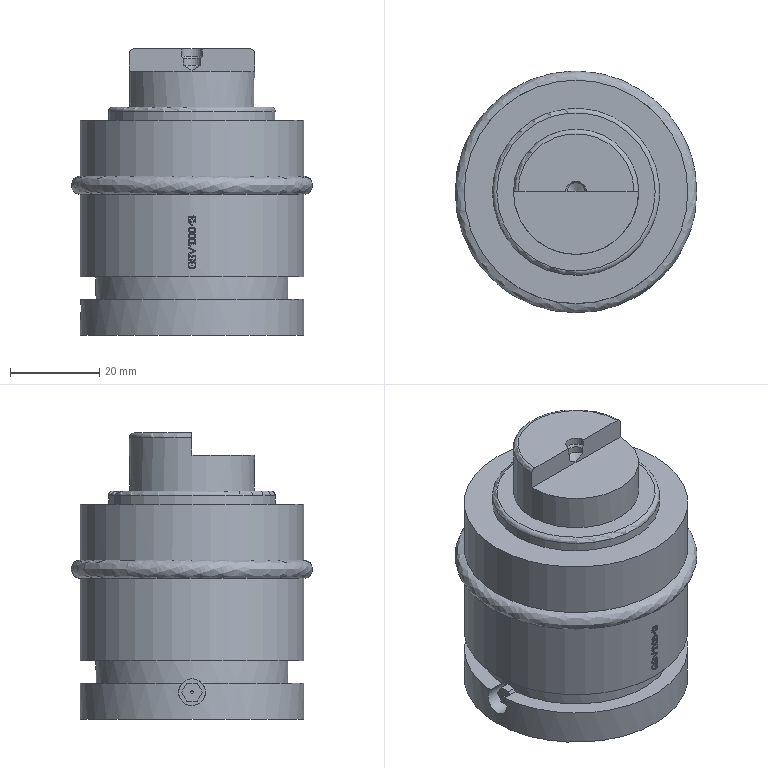Part | NX | features solid 2 | 1 solid | 181 faces | box 54.1 x 54.1 x 64 mm | volume 101548 mm3 | plane 92 | cylinder 80 | cone 6 | torus 2 | spline 1 | commonest cylinder face diameters 49.8 x10 50 x6 0.728 x3 0.869 x3 0.872 x3 0.882 x3